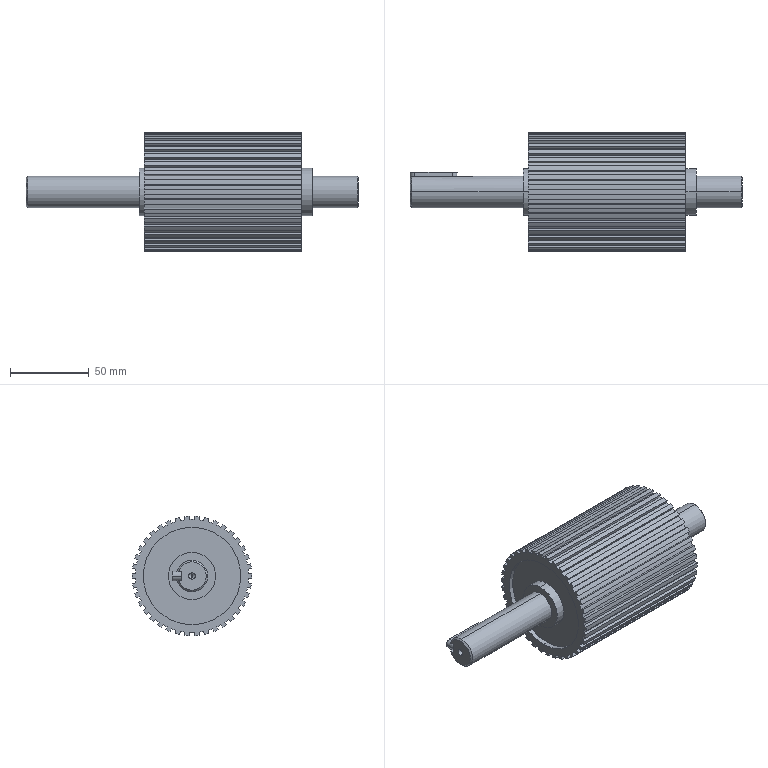Part | SolidWorks | 3 solids | 209 faces | box 211 x 76 x 75.929 mm | volume 292189 mm3 | cylinder 104 | plane 95 | cone 9 | spline 1 | commonest cylinder face diameters 72 x39 76 x38 62 x8 30 x6 4.2 x4 20 x4